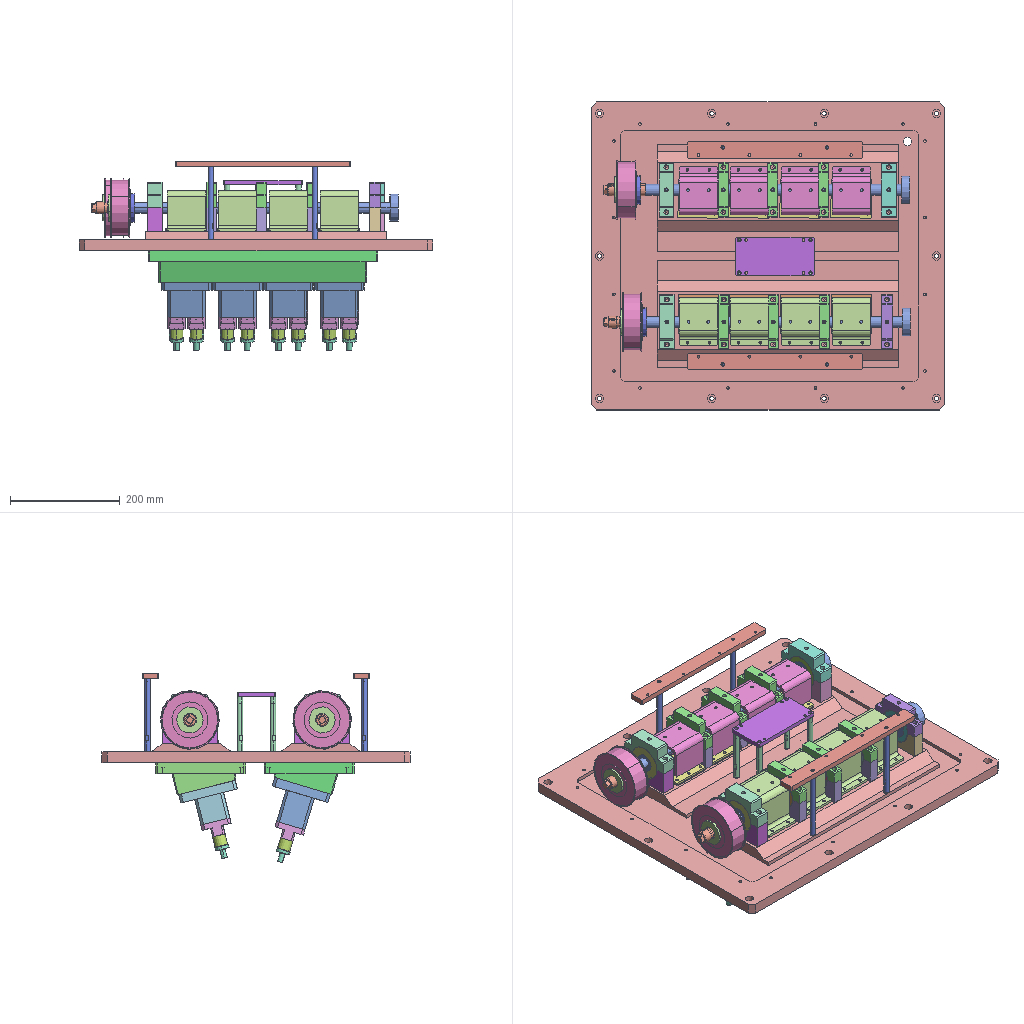Assembly | SolidWorks | 52 different items | 181 placed | box 645 x 562 x 346 mm
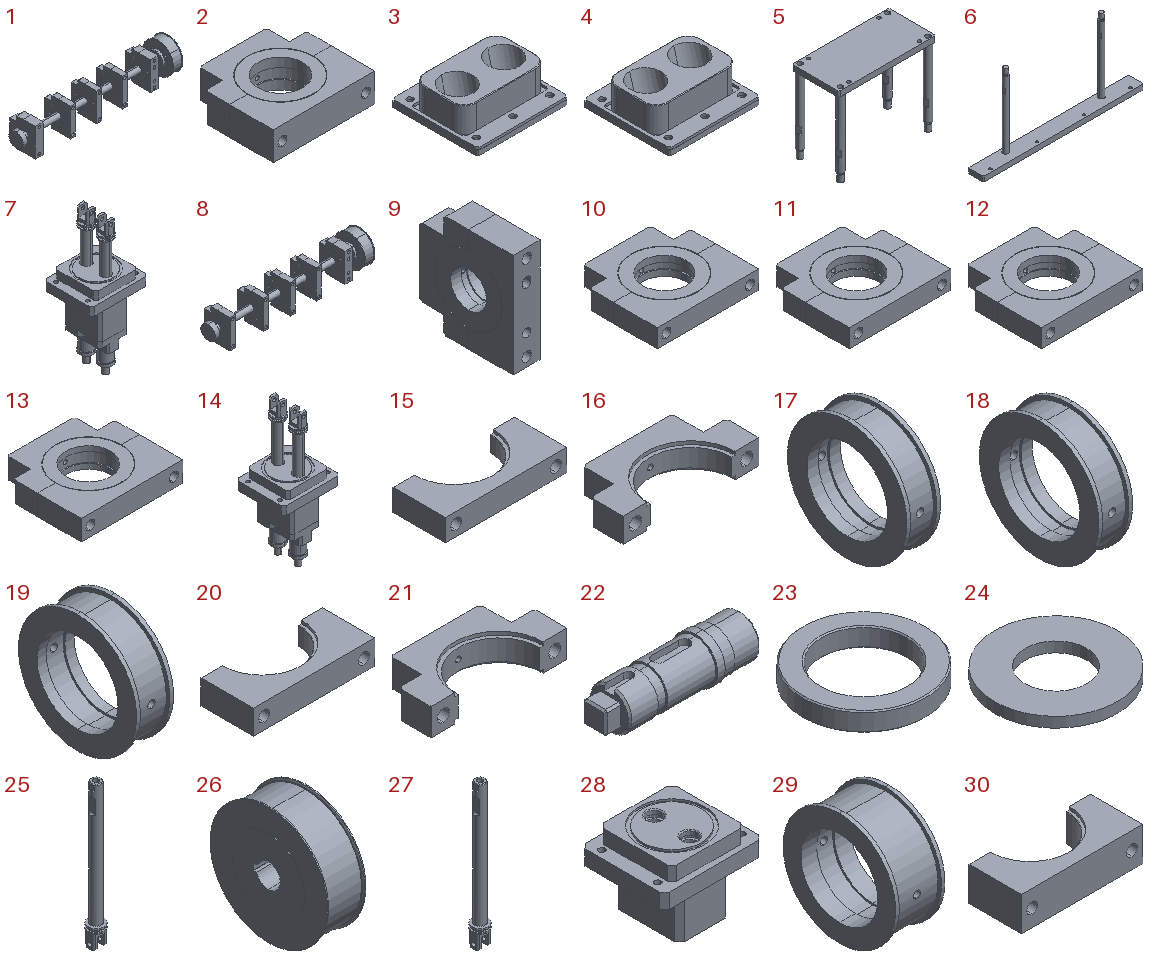Parts list (item | name | quantity | parent item | size | volume | features):
1 | (subassembly) | x1 | - | 559.6 x 107 x 107 mm | 1279109 mm3 | -
2 | (subassembly) | x1 | in 1 | 100 x 90 x 28 mm | 176248 mm3 | -
3 | (subassembly) | x4 | - | 74 x 70 x 25 mm | 56741 mm3 | -
4 | (subassembly) | x4 | - | 74 x 70 x 25 mm | 56433 mm3 | -
5 | (subassembly) | x1 | - | 144 x 70 x 121 mm | 111173 mm3 | features ReferencePattern 3, LocalLPattern 1
6 | (subassembly) | x2 | - | 320 x 30 x 156.2 mm | 116135 mm3 | features LocalLPattern 1, ReferencePattern 1
7 | (subassembly) | x4 | - | 106 x 90 x 252 mm | 546478 mm3 | -
8 | (subassembly) | x1 | - | 559.6 x 107 x 107 mm | 1225428 mm3 | -
9 | (subassembly) | x2 | in 1, 8 | 26 x 90 x 100 mm | 177639 mm3 | -
10 | (subassembly) | x2 | in 1, 8 | 100 x 90 x 18 mm | 110821 mm3 | -
11 | (subassembly) | x2 | in 1, 8 | 100 x 90 x 18 mm | 110453 mm3 | -
12 | (subassembly) | x2 | in 1, 8 | 100 x 90 x 18 mm | 110082 mm3 | -
13 | (subassembly) | x1 | in 8 | 100 x 90 x 20 mm | 122567 mm3 | -
14 | (subassembly) | x4 | - | 106 x 90 x 252 mm | 513009 mm3 | -
15 | - | x6 | in 10, 11, 12 | 100 x 43 x 18 mm | 45196 mm3 | features HoleWzd 2, ICE 2, Chamfer 1, Extrusion 1
16 | - | x6 | in 10, 11, 12 | 100 x 47 x 18 mm | 40091 mm3 | features HoleWzd 3, ICE 2, Chamfer 1, Extrusion 1
17 | - | x2 | in 11 | 18 x 64 x 64 mm | 25166 mm3 | features HoleWzd 3, Fillet 2, Revolution 1
18 | - | x2 | in 12 | 18 x 64 x 64 mm | 24795 mm3 | features HoleWzd 3, Fillet 2, Revolution 1
19 | - | x1 | in 13 | 20 x 64 x 64 mm | 26515 mm3 | features HoleWzd 3, Fillet 2, Revolution 1
20 | - | x1 | in 13 | 100 x 43 x 20 mm | 50968 mm3 | features HoleWzd 2, ICE 2, Chamfer 1, Extrusion 1
21 | - | x1 | in 13 | 100 x 47 x 20 mm | 45084 mm3 | features HoleWzd 3, ICE 2, Chamfer 1, Extrusion 1
22 | - | x2 | in 1, 8 | 77.5 x 24 x 24 mm | 26951 mm3 | features ICE 3, Chamfer 1, Revolution 1
23 | - | x2 | in 1, 8 | 52 x 52 x 8 mm | 8778 mm3 | features Chamfer 1, Extrusion 1
24 | - | x2 | in 1, 8 | 48 x 48 x 4 mm | 5429 mm3 | features Extrusion 1
25 | - | x8 | in 7 | 25 x 25 x 229 mm | 45704 mm3 | features ICE 7, Fillet 3, HoleWzd 3, Chamfer 1, Extrusion 1, RevCut 1
26 | - | x2 | in 1, 8 | 36 x 107 x 107 mm | 274839 mm3 | features ICE 3, Fillet 1, Revolution 1
27 | - | x8 | in 14 | 25 x 25 x 229 mm | 45697 mm3 | features ICE 7, Fillet 3, HoleWzd 3, Chamfer 1, Extrusion 1, RevCut 1
28 | - | x4 | in 14 | 106 x 90 x 79 mm | 359467 mm3 | features HoleWzd 4, ICE 4, Chamfer 2, Extrusion 1
29 | - | x1 | in 2 | 28 x 64 x 64 mm | 37136 mm3 | features HoleWzd 3, Fillet 2, Revolution 1
30 | - | x1 | in 2 | 100 x 43 x 28 mm | 74059 mm3 | features HoleWzd 2, ICE 2, Chamfer 1, Extrusion 1
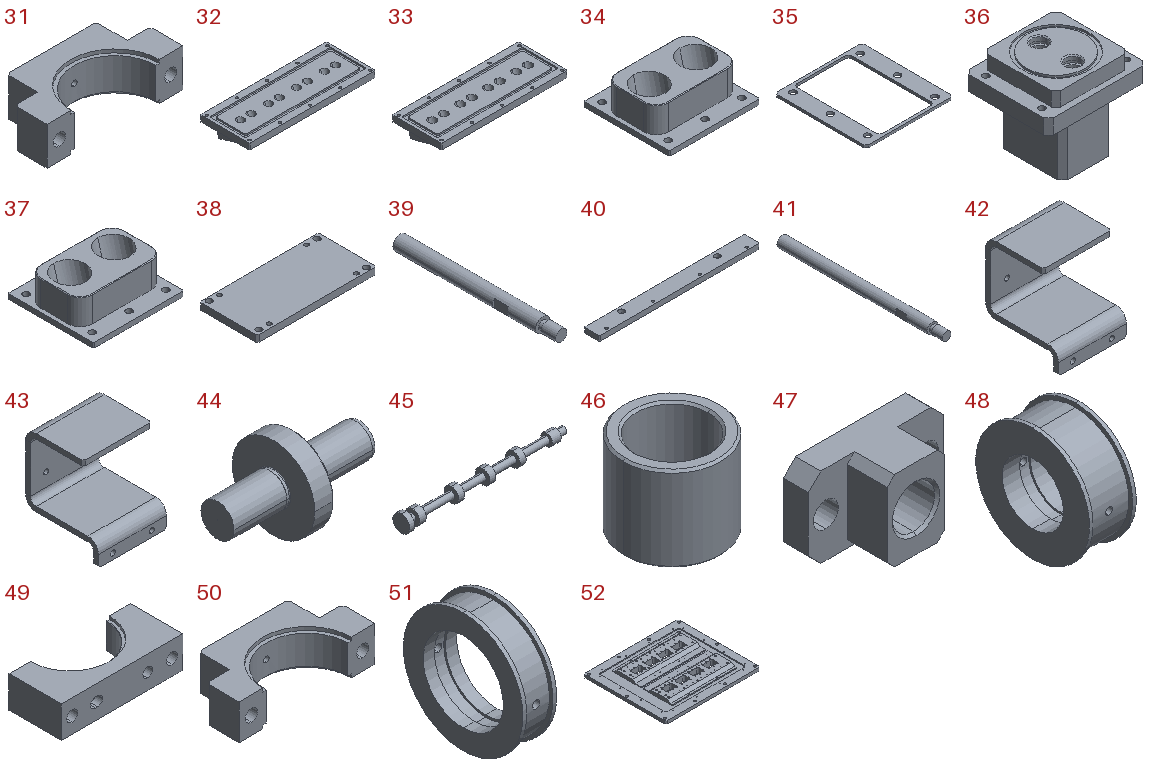31 | - | x1 | in 2 | 100 x 47 x 28 mm | 65054 mm3 | features HoleWzd 3, ICE 2, Chamfer 1, Extrusion 1
32 | - | x1 | - | 419 x 164 x 57.82 mm | 1739257 mm3 | features HoleWzd 3, ICE 3, Chamfer 2, Fillet 2, Extrusion 1
33 | - | x1 | - | 419 x 164 x 58.51 mm | 1832163 mm3 | features HoleWzd 3, ICE 3, Chamfer 2, Fillet 2, Extrusion 1
34 | - | x4 | in 3 | 74 x 70 x 25 mm | 52689 mm3 | features Chamfer 2, Extrusion 1, ICE 1, MirrorPattern 1, SweepCut 1
35 | - | x8 | in 3, 4 | 70 x 74 x 2 mm | 4052 mm3 | features Chamfer 1, Extrusion 1
36 | - | x4 | in 7 | 106 x 90 x 91 mm | 392922 mm3 | features HoleWzd 4, ICE 4, Chamfer 2, Extrusion 1
37 | - | x4 | in 4 | 74 x 70 x 25 mm | 52381 mm3 | features Chamfer 2, Extrusion 1, ICE 1, MirrorPattern 1, SweepCut 1
38 | - | x1 | in 5 | 144 x 70 x 8 mm | 78716 mm3 | features Chamfer 1, Extrusion 1, HoleWzd 1
39 | - | x4 | in 5 | 10 x 113 x 10 mm | 8114 mm3 | features HoleWzd 1, ICE 1, Revolution 1
40 | - | x2 | in 6 | 320 x 30 x 10 mm | 93623 mm3 | features HoleWzd 2, Chamfer 1, Extrusion 1
41 | - | x4 | in 6 | 10 x 153 x 10 mm | 11256 mm3 | features HoleWzd 1, ICE 1, Revolution 1
42 | - | x4 | - | 70 x 75 x 88 mm | 70287 mm3 | features EdgeFlange 3, HoleWzd 2, Chamfer 1, FlatPattern 1, SMBaseFlange 1, SheetMetal 1
43 | - | x4 | - | 70 x 75 x 88 mm | 70287 mm3 | features EdgeFlange 3, HoleWzd 2, Chamfer 1, FlatPattern 1, SMBaseFlange 1, SheetMetal 1
44 | - | x16 | in 7, 14 | 43 x 25 x 25 mm | 5837 mm3 | features ICE 5, RevCut 5, Revolution 4, Fillet 2, Chamfer 1, DelFace 1, RefAxis 1
45 | - | x2 | in 1, 8 | 482.1 x 50 x 50 mm | 277870 mm3 | features Revolution 1
46 | - | x16 | in 7, 14 | 23 x 23 x 20 mm | 3738 mm3 | features Chamfer 1, Extrusion 1
47 | - | x16 | in 7, 14 | 54 x 29 x 32 mm | 21498 mm3 | features Chamfer 4, HoleWzd 2, Extrusion 1, ICE 1
48 | - | x2 | in 9 | 26 x 64.446 x 64.446 mm | 49939 mm3 | features HoleWzd 3, Fillet 2, Revolution 1
49 | - | x2 | in 9 | 100 x 43 x 26 mm | 67587 mm3 | features HoleWzd 3, ICE 3, Chamfer 1, Extrusion 1
50 | - | x2 | in 9 | 100 x 47 x 26 mm | 60113 mm3 | features HoleWzd 3, ICE 2, Chamfer 1, Extrusion 1
51 | - | x2 | in 10 | 18 x 64 x 64 mm | 25534 mm3 | features HoleWzd 3, Fillet 2, Revolution 1
52 | - | x1 | - | 645 x 562 x 35 mm | 7508187 mm3 | features HoleWzd 10, ICE 3, Chamfer 1, Extrusion 1, Fillet 1
Mates (type | each side: item.copy, entity, surface, feature):
In the top assembly
Coincident | 52.1 face plane Boss-Extrude2 | 49.1 face plane Boss-Extrude1
Concentric | 52.1 face cylinder M8 Tapped Hole2 | 31.1 face cylinder Hole2 | 2 times
Concentric | 52.1 face cylinder M8 Tapped Hole2 | 49.2 face cylinder Hole1 | 2 times
Coincident | 52.1 face plane Boss-Extrude2 | 49.2 face plane Boss-Extrude1
Concentric | 52.1 face cylinder M8 Tapped Hole1 | 32.1 face cylinder Hole1 | 2 times
Coincident | 52.1 face plane Boss-Extrude1 | 32.1 face plane Boss-Extrude1
Concentric | 32.1 face cylinder Hole2 | 25.1 face cylinder Boss-Extrude1
Concentric | 32.1 face cylinder Hole2 | 25.2 face cylinder Boss-Extrude1
Coincident | 32.1 face plane Boss-Extrude2 | 36.1 face plane Boss-Extrude2
Concentric | 25.1 face cylinder Boss-Extrude1 | 37.1 face cylinder Cut-Sweep2
Concentric | 25.2 face cylinder Boss-Extrude1 | 37.1 face cylinder Mirror3
Coincident | 52.1 face plane Boss-Extrude2 | 35.1 face plane Boss-Extrude1
Concentric | 52.1 face cylinder M8 Tapped Hole1 | 33.1 face cylinder Hole1 | 2 times
Coincident | 52.1 face plane Boss-Extrude1 | 33.1 face plane Boss-Extrude1
Concentric | 33.1 face cylinder Hole2 | 27.1 face cylinder Boss-Extrude1
Concentric | 33.1 face cylinder Hole2 | 27.2 face cylinder Boss-Extrude1
Coincident | 33.1 face plane Boss-Extrude2 | 28.1 face plane Boss-Extrude2
Concentric | 27.2 face cylinder Boss-Extrude1 | 34.1 face cylinder Mirror1
Concentric | 27.1 face cylinder Boss-Extrude1 | 34.1 face cylinder Cut-Sweep1
Concentric | 52.1 face cylinder M6 Tapped Hole2 | 39.1 face cylinder Revolve1
Concentric | 52.1 face cylinder M6 Tapped Hole2 | 39.2 face cylinder Revolve1
Coincident | 52.1 face plane Boss-Extrude2 | 39.1 face plane Revolve1
Concentric | 52.1 face cylinder M8 Tapped Hole3 | 41.1 face cylinder Revolve1
Concentric | 52.1 face cylinder M8 Tapped Hole3 | 41.2 face cylinder Revolve1
Coincident | 52.1 face plane Boss-Extrude2 | 41.1 face plane Revolve1
Concentric | 52.1 face cylinder M8 Tapped Hole3 | 41.3 face cylinder Revolve1
Concentric | 52.1 face cylinder M8 Tapped Hole3 | 41.4 face cylinder Revolve1
Coincident | 52.1 face plane Boss-Extrude2 | 41.4 face plane Revolve1
Concentric | 52.1 face cylinder M4 Tapped Hole1 | 42.1 face cylinder Hole2 | 2 times
Coincident | 52.1 face plane Boss-Extrude2 | 42.1 face plane Edge-Flange3
Concentric | 52.1 face cylinder M4 Tapped Hole1 | 43.1 face cylinder Hole2 | 2 times
Coincident | 52.1 face plane Boss-Extrude2 | 43.1 face plane Edge-Flange3
In subassembly 1
Concentric | 45.1 face cylinder Revolve1 | 29.1 face cylinder Revolve1
Coincident | 45.1 face plane Revolve1 | 29.1 face plane Revolve1
Concentric | 45.1 face cylinder Revolve1 | 18.1 face cylinder Revolve1
Coincident | 45.1 face plane Revolve1 | 16.1 face plane Boss-Extrude1
Concentric | 45.1 face cylinder Revolve1 | 17.1 face cylinder Revolve1
Coincident | 45.1 face plane Revolve1 | 15.1 face plane Boss-Extrude1
Concentric | 45.1 face cylinder Revolve1 | 51.1 face cylinder Revolve1
Coincident | 45.1 face plane Revolve1 | 15.2 face plane Boss-Extrude1
Coincident | 45.1 face plane Revolve1 | 48.1 face plane Revolve1
Concentric | 45.1 face cylinder Revolve1 | 48.1 face cylinder Revolve1
Coincident | 31.2 face plane Boss-Extrude1 | 16.1 face plane Boss-Extrude1
Coincident | 16.2 face plane Boss-Extrude1 | 16.1 face plane Boss-Extrude1
Coincident | 16.3 face plane Boss-Extrude1 | 16.2 face plane Boss-Extrude1
Coincident | 16.3 face plane Boss-Extrude1 | 50.1 face plane Boss-Extrude1
Coincident | 24.1 face plane Boss-Extrude1 | 26.1 face plane Revolve1
Coincident | 23.1 face plane Boss-Extrude1 | 26.1 face plane Revolve1
Concentric | 23.1 face cylinder Boss-Extrude1 | 26.1 face cylinder Cut-Extrude2
Concentric | 45.1 face cylinder Revolve1 | 26.1 face cylinder Cut-Extrude2
Concentric | 24.1 face cylinder Boss-Extrude1 | 26.1 face cylinder Cut-Extrude1
Concentric | 22.1 face cylinder Revolve1 | 26.1 face cylinder Cut-Extrude3
Parallel | 22.1 face plane Cut-Extrude1 | 26.1 face plane Cut-Extrude2
Coincident | 45.1 face plane Revolve1 | 22.1 face plane Revolve1
In subassembly 12
Concentric | 16.4 face cylinder M8x1.0 Tapped Hole1 | 18.2 face cylinder Hole1
Concentric | 16.4 face cylinder Boss-Extrude1 | 18.2 face cylinder Revolve1
Concentric | 15.3 face cylinder Boss-Extrude1 | 18.2 face cylinder Revolve1
Coincident | 16.4 face plane Boss-Extrude1 | 18.2 face plane Revolve1
Coincident | 15.3 face plane Boss-Extrude1 | 18.2 face plane Revolve1
Coincident | 15.3 face plane Boss-Extrude1 | 16.4 face plane Boss-Extrude1
In subassembly 2
Concentric | 29.2 face cylinder Hole2 | 31.3 face cylinder M8x1.0 Tapped Hole1
Concentric | 29.2 face cylinder Revolve1 | 31.3 face cylinder Boss-Extrude1
Concentric | 29.2 face cylinder Revolve1 | 30.1 face cylinder Boss-Extrude1
Coincident | 30.1 face plane Boss-Extrude1 | 31.3 face plane Boss-Extrude1 | 2 times
Coincident | 29.2 face plane Revolve1 | 31.3 face plane Boss-Extrude1
In subassembly 10
Concentric | 51.2 face cylinder Hole2 | 16.4 face cylinder M8x1.0 Tapped Hole1
Concentric | 51.2 face cylinder Revolve1 | 16.4 face cylinder Boss-Extrude1
Concentric | 51.2 face cylinder Revolve1 | 15.3 face cylinder Boss-Extrude1
Coincident | 15.3 face plane Boss-Extrude1 | 16.4 face plane Boss-Extrude1 | 2 times
In subassembly 11
Concentric | 16.4 face cylinder M8x1.0 Tapped Hole1 | 17.2 face cylinder Hole1
Concentric | 16.4 face cylinder Boss-Extrude1 | 17.2 face cylinder Revolve1
Concentric | 15.3 face cylinder Boss-Extrude1 | 17.2 face cylinder Revolve1
Coincident | 16.4 face plane Boss-Extrude1 | 17.2 face plane Revolve1
Coincident | 15.3 face plane Boss-Extrude1 | 17.2 face plane Revolve1
Coincident | 15.3 face plane Boss-Extrude1 | 16.4 face plane Boss-Extrude1
In subassembly 9
Coincident | 49.3 face plane Boss-Extrude1 | 50.2 face plane Boss-Extrude1 | 2 times
Concentric | 48.2 face cylinder Revolve1 | 50.2 face cylinder Boss-Extrude1
Coincident | 48.2 face plane Revolve1 | 49.3 face plane Boss-Extrude1
Concentric | 48.2 face cylinder Revolve1 | 49.3 face cylinder Boss-Extrude1
Parallel | 49.3 face plane Boss-Extrude1 | 9.1 plane
Concentric | 48.2 face cylinder Hole2 | 50.2 face cylinder M8x1.0 Tapped Hole1
In subassembly 8
Concentric | 45.1 face cylinder Revolve1 | 48.1 face cylinder Revolve1
Concentric | 45.1 face cylinder Revolve1 | 51.1 face cylinder Revolve1
Concentric | 45.1 face cylinder Revolve1 | 17.1 face cylinder Revolve1
Concentric | 45.1 face cylinder Revolve1 | 18.1 face cylinder Revolve1
Concentric | 45.1 face cylinder Revolve1 | 19.1 face cylinder Revolve1
Coincident | 15.4 face plane Boss-Extrude1 | 20.1 face plane Boss-Extrude1
Coincident | 15.1 face plane Boss-Extrude1 | 15.4 face plane Boss-Extrude1
Coincident | 15.2 face plane Boss-Extrude1 | 15.1 face plane Boss-Extrude1
Coincident | 49.4 face plane Boss-Extrude1 | 15.2 face plane Boss-Extrude1
Coincident | 45.1 face plane Revolve1 | 19.1 face plane Revolve1
Coincident | 45.1 face plane Revolve1 | 18.1 face plane Revolve1
Coincident | 45.1 face plane Revolve1 | 16.2 face plane Boss-Extrude1
Coincident | 45.1 face plane Revolve1 | 15.2 face plane Boss-Extrude1
Coincident | 45.1 face plane Revolve1 | 50.1 face plane Boss-Extrude1
Parallel | 22.1 face plane Cut-Extrude1 | 26.1 face plane Cut-Extrude2
Concentric | 22.1 face cylinder Revolve1 | 26.1 face cylinder Cut-Extrude1
Concentric | 22.1 face cylinder Revolve1 | 23.1 face cylinder Boss-Extrude1
Coincident | 23.1 face plane Boss-Extrude1 | 26.1 face plane Revolve1
Coincident | 24.1 face plane Boss-Extrude1 | 26.1 face plane Revolve1
Concentric | 22.1 face cylinder Revolve1 | 24.1 face cylinder Boss-Extrude1
Concentric | 45.1 face cylinder Revolve1 | 22.1 face cylinder Revolve1
Coincident | 45.1 face plane Revolve1 | 22.1 face plane Revolve1
In subassembly 13
Concentric | 19.2 face cylinder Hole2 | 21.1 face cylinder M8x1.0 Tapped Hole1
Concentric | 19.2 face cylinder Revolve1 | 21.1 face cylinder Boss-Extrude1
Concentric | 19.2 face cylinder Revolve1 | 20.2 face cylinder Boss-Extrude1
Coincident | 19.2 face plane Revolve1 | 20.2 face plane Boss-Extrude1
Coincident | 20.2 face plane Boss-Extrude1 | 21.1 face plane Boss-Extrude1
In subassembly 4
Coincident | 37.2 face plane Boss-Extrude1 | 35.2 face plane Boss-Extrude1 | 3 times
In subassembly 14
Coincident | 27.3 face plane Cut-Extrude1 | 27.4 face plane Cut-Extrude1
Coincident | 27.3 face plane Cut-Extrude3 | 27.4 face plane Cut-Extrude3
Concentric | 27.3 face cylinder Boss-Extrude1 | 47.1 face cylinder Hole3 | 2 times
Coincident | 28.2 face plane Boss-Extrude1 | 47.1 face plane Boss-Extrude1
Concentric | 27.4 face cylinder Boss-Extrude1 | 47.2 face cylinder Hole3
Coincident | 28.2 face plane Boss-Extrude1 | 47.2 face plane Boss-Extrude1
Concentric | 27.4 face cylinder Boss-Extrude1 | 46.1 face cylinder Boss-Extrude1
Concentric | 27.3 face cylinder Boss-Extrude1 | 46.2 face cylinder Boss-Extrude1
Coincident | 46.1 face plane Boss-Extrude1 | 47.2 face plane Boss-Extrude1
Coincident | 46.2 face plane Boss-Extrude1 | 47.1 face plane Boss-Extrude1
Coincident | 27.4 face plane Boss-Extrude1 | 46.1 face plane Boss-Extrude1
Coincident | 46.1 face plane Boss-Extrude1 | 44.1 face plane Revolve1
Concentric | 46.1 face cylinder Boss-Extrude1 | 44.1 face cylinder Revolve1
Coincident | 46.2 face plane Boss-Extrude1 | 44.2 face plane Revolve1
Concentric | 46.2 face cylinder Boss-Extrude1 | 44.2 face cylinder Revolve1
Concentric | 28.2 face cylinder Hole1 | 27.4 face cylinder Boss-Extrude1
Concentric | 27.3 face cylinder Boss-Extrude1 | 28.2 face cylinder Hole2
Concentric | 28.2 face cylinder M5 Tapped Hole1 | 47.2 face cylinder Hole2 | 2 times
Concentric | 28.2 face cylinder M5 Tapped Hole1 | 47.1 face cylinder Hole2 | 2 times
In subassembly 3
Coincident | 34.2 face plane Boss-Extrude1 | 35.2 face plane Boss-Extrude1 | 3 times
In subassembly 6
Concentric | 40.1 face cylinder Hole1 | 41.5 face cylinder Revolve1
Coincident | 40.1 face plane Hole1 | 41.5 face plane Revolve1
In subassembly 7
Concentric | 25.3 face cylinder Boss-Extrude1 | 36.2 face cylinder Hole1
Concentric | 25.4 face cylinder Boss-Extrude1 | 36.2 face cylinder Hole1
Coincident | 25.3 face plane Cut-Extrude1 | 25.4 face plane Cut-Extrude1
Coincident | 25.3 face plane Cut-Extrude3 | 25.4 face plane Cut-Extrude3
Parallel | 25.4 face plane Cut-Extrude3 | 36.2 face plane Boss-Extrude3
Concentric | 36.2 face cylinder M5 Tapped Hole1 | 47.2 face cylinder Hole2 | 2 times
Concentric | 36.2 face cylinder M5 Tapped Hole1 | 47.1 face cylinder Hole2 | 2 times
Coincident | 36.2 face plane Boss-Extrude1 | 47.1 face plane Boss-Extrude1
Coincident | 36.2 face plane Boss-Extrude1 | 47.2 face plane Boss-Extrude1
Concentric | 25.3 face cylinder Boss-Extrude1 | 46.1 face cylinder Boss-Extrude1
Concentric | 25.4 face cylinder Boss-Extrude1 | 46.2 face cylinder Boss-Extrude1
Coincident | 46.1 face plane Boss-Extrude1 | 47.2 face plane Boss-Extrude1
Coincident | 46.2 face plane Boss-Extrude1 | 47.1 face plane Boss-Extrude1
Coincident | 25.3 face plane Boss-Extrude1 | 46.1 face plane Boss-Extrude1
Concentric | 25.3 face cylinder Hole2 | 44.1 face cylinder Revolve1
Coincident | 46.1 face plane Boss-Extrude1 | 44.1 face plane Revolve1
Coincident | 44.1 face plane Revolve1 | 44.2 face plane Revolve1
Concentric | 25.4 face cylinder Hole2 | 44.2 face cylinder Revolve1
In subassembly 5
Concentric | 38.1 face cylinder Boss-Extrude1 | 39.3 face cylinder Revolve1
Coincident | 38.1 face plane Boss-Extrude1 | 39.3 face plane Revolve1